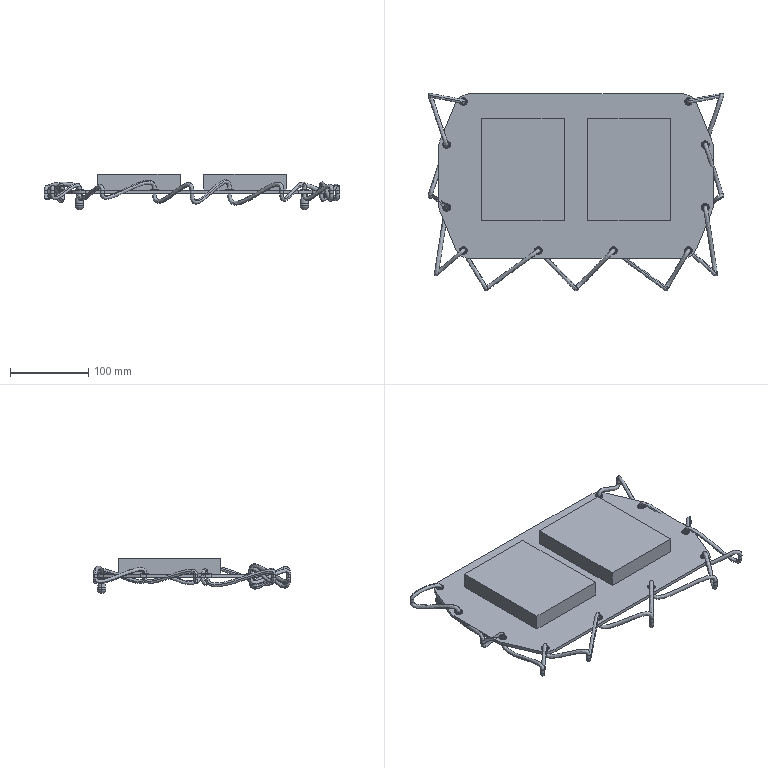Part | SolidWorks | 25 solids | 366 faces | box 377.126 x 251.517 x 45 mm | volume 856540 mm3 | cylinder 154 | torus 84 | plane 70 | spline 38 | cone 12 | sphere 8 | commonest cylinder face diameters 6 x60 10 x40 5 x38 40 x8 7.8 x4 9.2 x4